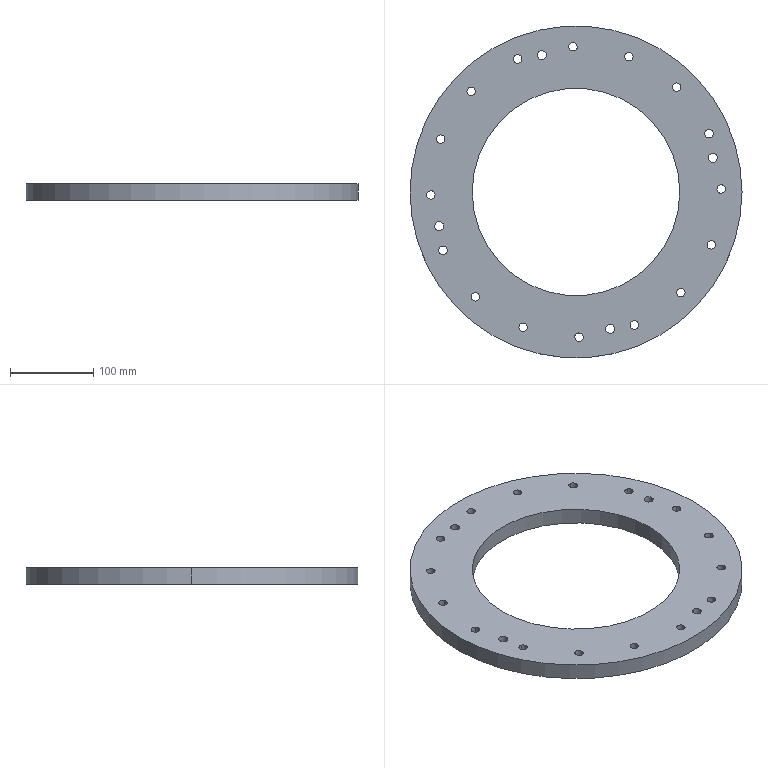Part | SolidWorks | features CirPattern 2, HoleWzd 2, Extrusion 1, ICE 1 | 1 solid | 58 faces | box 400 x 400 x 20 mm | volume 1490760 mm3 | cylinder 52 | plane 6 | commonest cylinder face diameters 10.2 x32 11 x8 18 x8 250 x2 400 x2